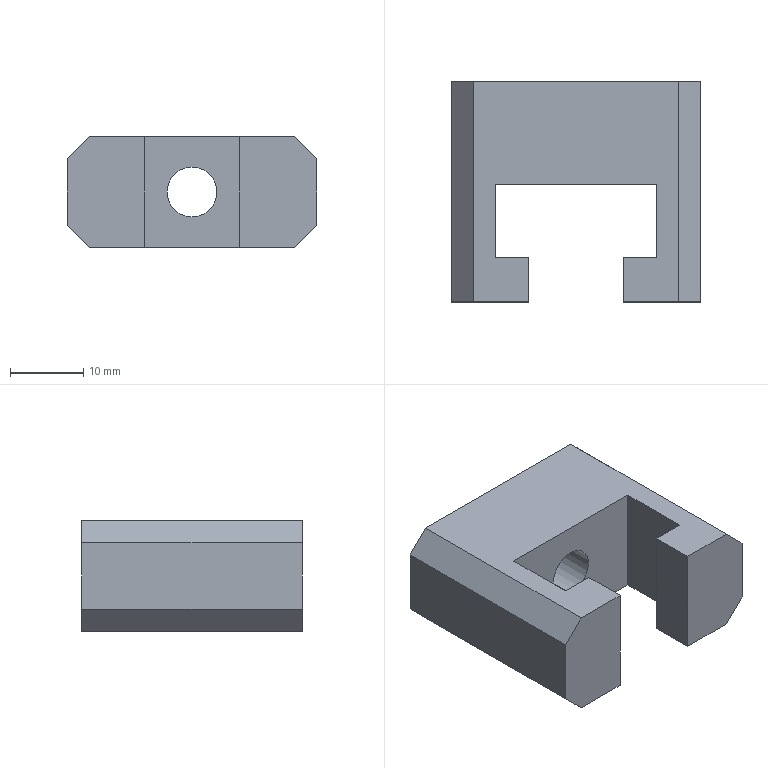Part | STEP file | union 1 | 1 solid | 20 faces | box 34 x 30 x 15 mm | volume 9782 mm3 | plane 18 | cylinder 2 | commonest cylinder face diameters 6.8 x2
STEP:
#1=CARTESIAN_POINT('',(0.,0.,0.));
#2=DIRECTION('',(0.,0.,1.));
#3=DIRECTION('',(1.,0.,0.));
#4=AXIS2_PLACEMENT_3D('',#1,#2,#3);
#5=CARTESIAN_POINT('',(17.,16.,10.9));
#6=VERTEX_POINT('',#5);
#7=CARTESIAN_POINT('',(17.,30.,10.9));
#8=VERTEX_POINT('',#7);
#9=CARTESIAN_POINT('',(17.,30.,10.9));
#10=DIRECTION('',(0.,1.,0.));
#11=VECTOR('',#10,1.);
#12=LINE('',#9,#11);
#13=CARTESIAN_POINT('',(17.,30.,7.5));
#14=DIRECTION('',(0.,1.,0.));
#15=DIRECTION('',(0.,0.,1.));
#16=AXIS2_PLACEMENT_3D('',#13,#14,#15);
#17=CYLINDRICAL_SURFACE('',#16,3.4);
#18=CARTESIAN_POINT('',(6.283,0.));
#19=DIRECTION('',(0.,1.));
#20=VECTOR('',#19,1.);
#21=LINE('',#18,#20);
#22=(GEOMETRIC_REPRESENTATION_CONTEXT(2)PARAMETRIC_REPRESENTATION_CONTEXT()REPRESENTATION_CONTEXT('',''));
#23=DEFINITIONAL_REPRESENTATION('',(#21),#22);
#24=PCURVE('',#17,#23);
#25=CARTESIAN_POINT('',(17.,30.,7.5));
#26=DIRECTION('',(0.,1.,0.));
#27=DIRECTION('',(0.,0.,1.));
#28=AXIS2_PLACEMENT_3D('',#25,#26,#27);
#29=CYLINDRICAL_SURFACE('',#28,3.4);
#30=CARTESIAN_POINT('',(0.,0.));
#31=DIRECTION('',(0.,1.));
#32=VECTOR('',#31,1.);
#33=LINE('',#30,#32);
#34=(GEOMETRIC_REPRESENTATION_CONTEXT(2)PARAMETRIC_REPRESENTATION_CONTEXT()REPRESENTATION_CONTEXT('',''));
#35=DEFINITIONAL_REPRESENTATION('',(#33),#34);
#36=PCURVE('',#29,#35);
#37=SURFACE_CURVE('',#12,(#24,#36),.PCURVE_S1.);
#38=EDGE_CURVE('',#6,#8,#37,.T.);
#39=ORIENTED_EDGE('',*,*,#38,.T.);
#40=CARTESIAN_POINT('',(17.,30.,4.1));
#41=VERTEX_POINT('',#40);
#42=CARTESIAN_POINT('',(17.,30.,7.5));
#43=DIRECTION('',(0.,1.,0.));
#44=DIRECTION('',(0.,0.,1.));
#45=AXIS2_PLACEMENT_3D('',#42,#43,#44);
#46=CIRCLE('',#45,3.4);
#47=CARTESIAN_POINT('',(0.,0.));
#48=DIRECTION('',(1.,0.));
#49=VECTOR('',#48,1.);
#50=LINE('',#47,#49);
#51=(GEOMETRIC_REPRESENTATION_CONTEXT(2)PARAMETRIC_REPRESENTATION_CONTEXT()REPRESENTATION_CONTEXT('',''));
#52=DEFINITIONAL_REPRESENTATION('',(#50),#51);
#53=PCURVE('',#17,#52);
#54=CARTESIAN_POINT('',(0.,30.,15.));
#55=DIRECTION('',(0.,-1.,0.));
#56=DIRECTION('',(1.,0.,0.));
#57=AXIS2_PLACEMENT_3D('',#54,#55,#56);
#58=PLANE('',#57);
#59=CARTESIAN_POINT('',(17.,-4.1));
#60=CARTESIAN_POINT('',(22.889,-4.1));
#61=CARTESIAN_POINT('',(19.944,-9.2));
#62=CARTESIAN_POINT('',(17.,-14.3));
#63=CARTESIAN_POINT('',(14.056,-9.2));
#64=CARTESIAN_POINT('',(11.111,-4.1));
#65=CARTESIAN_POINT('',(17.,-4.1));
#66=(BOUNDED_CURVE()B_SPLINE_CURVE(2,(#59,#60,#61,#62,#63,#64,#65),.UNSPECIFIED.,.T.,.F.)B_SPLINE_CURVE_WITH_KNOTS((1,2,2,2,2,1),(-2.094,0.,2.094,4.189,6.283,8.378),.UNSPECIFIED.)CURVE()GEOMETRIC_REPRESENTATION_ITEM()RATIONAL_B_SPLINE_CURVE((1.,0.5,1.,0.5,1.,0.5,1.))REPRESENTATION_ITEM(''));
#67=(GEOMETRIC_REPRESENTATION_CONTEXT(2)PARAMETRIC_REPRESENTATION_CONTEXT()REPRESENTATION_CONTEXT('',''));
#68=DEFINITIONAL_REPRESENTATION('',(#66),#67);
#69=PCURVE('',#58,#68);
#70=SURFACE_CURVE('',#46,(#53,#69),.PCURVE_S1.);
#71=EDGE_CURVE('',#41,#8,#70,.T.);
#72=ORIENTED_EDGE('',*,*,#71,.F.);
#73=CARTESIAN_POINT('',(17.,16.,4.1));
#74=VERTEX_POINT('',#73);
#75=CARTESIAN_POINT('',(17.,30.,4.1));
#76=DIRECTION('',(0.,1.,0.));
#77=VECTOR('',#76,1.);
#78=LINE('',#75,#77);
#79=CARTESIAN_POINT('',(3.142,0.));
#80=DIRECTION('',(0.,1.));
#81=VECTOR('',#80,1.);
#82=LINE('',#79,#81);
#83=(GEOMETRIC_REPRESENTATION_CONTEXT(2)PARAMETRIC_REPRESENTATION_CONTEXT()REPRESENTATION_CONTEXT('',''));
#84=DEFINITIONAL_REPRESENTATION('',(#82),#83);
#85=PCURVE('',#17,#84);
#86=CARTESIAN_POINT('',(3.142,0.));
#87=DIRECTION('',(0.,1.));
#88=VECTOR('',#87,1.);
#89=LINE('',#86,#88);
#90=(GEOMETRIC_REPRESENTATION_CONTEXT(2)PARAMETRIC_REPRESENTATION_CONTEXT()REPRESENTATION_CONTEXT('',''));
#91=DEFINITIONAL_REPRESENTATION('',(#89),#90);
#92=PCURVE('',#29,#91);
#93=SURFACE_CURVE('',#78,(#85,#92),.PCURVE_S1.);
#94=EDGE_CURVE('',#74,#41,#93,.T.);
#95=ORIENTED_EDGE('',*,*,#94,.F.);
#96=CARTESIAN_POINT('',(17.,16.,7.5));
#97=DIRECTION('',(0.,1.,0.));
#98=DIRECTION('',(-1.,0.,0.));
#99=AXIS2_PLACEMENT_3D('',#96,#97,#98);
#100=CIRCLE('',#99,3.4);
#101=CARTESIAN_POINT('',(-1.571,-14.));
#102=DIRECTION('',(1.,0.));
#103=VECTOR('',#102,1.);
#104=LINE('',#101,#103);
#105=(GEOMETRIC_REPRESENTATION_CONTEXT(2)PARAMETRIC_REPRESENTATION_CONTEXT()REPRESENTATION_CONTEXT('',''));
#106=DEFINITIONAL_REPRESENTATION('',(#104),#105);
#107=PCURVE('',#17,#106);
#108=CARTESIAN_POINT('',(6.,16.,15.));
#109=DIRECTION('',(0.,1.,0.));
#110=DIRECTION('',(-1.,0.,0.));
#111=AXIS2_PLACEMENT_3D('',#108,#109,#110);
#112=PLANE('',#111);
#113=CARTESIAN_POINT('',(-11.,-7.5));
#114=DIRECTION('',(1.,0.));
#115=AXIS2_PLACEMENT_2D('',#113,#114);
#116=CIRCLE('',#115,3.4);
#117=(GEOMETRIC_REPRESENTATION_CONTEXT(2)PARAMETRIC_REPRESENTATION_CONTEXT()REPRESENTATION_CONTEXT('',''));
#118=DEFINITIONAL_REPRESENTATION('',(#116),#117);
#119=PCURVE('',#112,#118);
#120=SURFACE_CURVE('',#100,(#107,#119),.PCURVE_S1.);
#121=EDGE_CURVE('',#74,#6,#120,.T.);
#122=ORIENTED_EDGE('',*,*,#121,.T.);
#123=EDGE_LOOP('',(#39,#72,#95,#122));
#124=FACE_BOUND('',#123,.F.);
#125=ADVANCED_FACE('',(#124),#17,.F.);
#126=CARTESIAN_POINT('',(0.,30.,12.));
#127=VERTEX_POINT('',#126);
#128=CARTESIAN_POINT('',(0.,30.,3.));
#129=VERTEX_POINT('',#128);
#130=CARTESIAN_POINT('',(0.,30.,15.));
#131=DIRECTION('',(0.,0.,-1.));
#132=VECTOR('',#131,1.);
#133=LINE('',#130,#132);
#134=CARTESIAN_POINT('',(0.,0.));
#135=DIRECTION('',(0.,-1.));
#136=VECTOR('',#135,1.);
#137=LINE('',#134,#136);
#138=(GEOMETRIC_REPRESENTATION_CONTEXT(2)PARAMETRIC_REPRESENTATION_CONTEXT()REPRESENTATION_CONTEXT('',''));
#139=DEFINITIONAL_REPRESENTATION('',(#137),#138);
#140=PCURVE('',#58,#139);
#141=CARTESIAN_POINT('',(0.,0.,15.));
#142=DIRECTION('',(1.,0.,0.));
#143=DIRECTION('',(0.,0.,-1.));
#144=AXIS2_PLACEMENT_3D('',#141,#142,#143);
#145=PLANE('',#144);
#146=CARTESIAN_POINT('',(0.,30.));
#147=DIRECTION('',(1.,0.));
#148=VECTOR('',#147,1.);
#149=LINE('',#146,#148);
#150=(GEOMETRIC_REPRESENTATION_CONTEXT(2)PARAMETRIC_REPRESENTATION_CONTEXT()REPRESENTATION_CONTEXT('',''));
#151=DEFINITIONAL_REPRESENTATION('',(#149),#150);
#152=PCURVE('',#145,#151);
#153=SURFACE_CURVE('',#133,(#140,#152),.PCURVE_S1.);
#154=EDGE_CURVE('',#127,#129,#153,.T.);
#155=ORIENTED_EDGE('',*,*,#154,.F.);
#156=CARTESIAN_POINT('',(3.,30.,15.));
#157=VERTEX_POINT('',#156);
#158=CARTESIAN_POINT('',(3.,30.,15.));
#159=DIRECTION('',(0.7071,0.,0.7071));
#160=VECTOR('',#159,1.);
#161=LINE('',#158,#160);
#162=CARTESIAN_POINT('',(3.,0.));
#163=DIRECTION('',(0.7071,0.7071));
#164=VECTOR('',#163,1.);
#165=LINE('',#162,#164);
#166=(GEOMETRIC_REPRESENTATION_CONTEXT(2)PARAMETRIC_REPRESENTATION_CONTEXT()REPRESENTATION_CONTEXT('',''));
#167=DEFINITIONAL_REPRESENTATION('',(#165),#166);
#168=PCURVE('',#58,#167);
#169=CARTESIAN_POINT('',(3.,0.,15.));
#170=DIRECTION('',(0.7071,0.,-0.7071));
#171=DIRECTION('',(-0.7071,0.,-0.7071));
#172=AXIS2_PLACEMENT_3D('',#169,#170,#171);
#173=PLANE('',#172);
#174=CARTESIAN_POINT('',(0.,30.));
#175=DIRECTION('',(-1.,0.));
#176=VECTOR('',#175,1.);
#177=LINE('',#174,#176);
#178=(GEOMETRIC_REPRESENTATION_CONTEXT(2)PARAMETRIC_REPRESENTATION_CONTEXT()REPRESENTATION_CONTEXT('',''));
#179=DEFINITIONAL_REPRESENTATION('',(#177),#178);
#180=PCURVE('',#173,#179);
#181=SURFACE_CURVE('',#161,(#168,#180),.PCURVE_S1.);
#182=EDGE_CURVE('',#127,#157,#181,.T.);
#183=ORIENTED_EDGE('',*,*,#182,.T.);
#184=CARTESIAN_POINT('',(31.,30.,15.));
#185=VERTEX_POINT('',#184);
#186=CARTESIAN_POINT('',(0.,30.,15.));
#187=DIRECTION('',(-1.,0.,0.));
#188=VECTOR('',#187,1.);
#189=LINE('',#186,#188);
#190=CARTESIAN_POINT('',(0.,0.));
#191=DIRECTION('',(-1.,0.));
#192=VECTOR('',#191,1.);
#193=LINE('',#190,#192);
#194=(GEOMETRIC_REPRESENTATION_CONTEXT(2)PARAMETRIC_REPRESENTATION_CONTEXT()REPRESENTATION_CONTEXT('',''));
#195=DEFINITIONAL_REPRESENTATION('',(#193),#194);
#196=PCURVE('',#58,#195);
#197=CARTESIAN_POINT('',(0.,0.,15.));
#198=DIRECTION('',(0.,0.,-1.));
#199=DIRECTION('',(-1.,0.,0.));
#200=AXIS2_PLACEMENT_3D('',#197,#198,#199);
#201=PLANE('',#200);
#202=CARTESIAN_POINT('',(0.,30.));
#203=DIRECTION('',(1.,0.));
#204=VECTOR('',#203,1.);
#205=LINE('',#202,#204);
#206=(GEOMETRIC_REPRESENTATION_CONTEXT(2)PARAMETRIC_REPRESENTATION_CONTEXT()REPRESENTATION_CONTEXT('',''));
#207=DEFINITIONAL_REPRESENTATION('',(#205),#206);
#208=PCURVE('',#201,#207);
#209=SURFACE_CURVE('',#189,(#196,#208),.PCURVE_S1.);
#210=EDGE_CURVE('',#185,#157,#209,.T.);
#211=ORIENTED_EDGE('',*,*,#210,.F.);
#212=CARTESIAN_POINT('',(34.,30.,12.));
#213=VERTEX_POINT('',#212);
#214=CARTESIAN_POINT('',(31.,30.,15.));
#215=DIRECTION('',(0.7071,0.,-0.7071));
#216=VECTOR('',#215,1.);
#217=LINE('',#214,#216);
#218=CARTESIAN_POINT('',(31.,0.));
#219=DIRECTION('',(0.7071,-0.7071));
#220=VECTOR('',#219,1.);
#221=LINE('',#218,#220);
#222=(GEOMETRIC_REPRESENTATION_CONTEXT(2)PARAMETRIC_REPRESENTATION_CONTEXT()REPRESENTATION_CONTEXT('',''));
#223=DEFINITIONAL_REPRESENTATION('',(#221),#222);
#224=PCURVE('',#58,#223);
#225=CARTESIAN_POINT('',(31.,0.,15.));
#226=DIRECTION('',(-0.7071,0.,-0.7071));
#227=DIRECTION('',(-0.7071,0.,0.7071));
#228=AXIS2_PLACEMENT_3D('',#225,#226,#227);
#229=PLANE('',#228);
#230=CARTESIAN_POINT('',(0.,30.));
#231=DIRECTION('',(-1.,0.));
#232=VECTOR('',#231,1.);
#233=LINE('',#230,#232);
#234=(GEOMETRIC_REPRESENTATION_CONTEXT(2)PARAMETRIC_REPRESENTATION_CONTEXT()REPRESENTATION_CONTEXT('',''));
#235=DEFINITIONAL_REPRESENTATION('',(#233),#234);
#236=PCURVE('',#229,#235);
#237=SURFACE_CURVE('',#217,(#224,#236),.PCURVE_S1.);
#238=EDGE_CURVE('',#185,#213,#237,.T.);
#239=ORIENTED_EDGE('',*,*,#238,.T.);
#240=CARTESIAN_POINT('',(34.,30.,3.));
#241=VERTEX_POINT('',#240);
#242=CARTESIAN_POINT('',(34.,30.,15.));
#243=DIRECTION('',(0.,0.,-1.));
#244=VECTOR('',#243,1.);
#245=LINE('',#242,#244);
#246=CARTESIAN_POINT('',(34.,0.));
#247=DIRECTION('',(0.,-1.));
#248=VECTOR('',#247,1.);
#249=LINE('',#246,#248);
#250=(GEOMETRIC_REPRESENTATION_CONTEXT(2)PARAMETRIC_REPRESENTATION_CONTEXT()REPRESENTATION_CONTEXT('',''));
#251=DEFINITIONAL_REPRESENTATION('',(#249),#250);
#252=PCURVE('',#58,#251);
#253=CARTESIAN_POINT('',(34.,0.,15.));
#254=DIRECTION('',(-1.,0.,0.));
#255=DIRECTION('',(0.,-1.,0.));
#256=AXIS2_PLACEMENT_3D('',#253,#254,#255);
#257=PLANE('',#256);
#258=CARTESIAN_POINT('',(-30.,0.));
#259=DIRECTION('',(0.,-1.));
#260=VECTOR('',#259,1.);
#261=LINE('',#258,#260);
#262=(GEOMETRIC_REPRESENTATION_CONTEXT(2)PARAMETRIC_REPRESENTATION_CONTEXT()REPRESENTATION_CONTEXT('',''));
#263=DEFINITIONAL_REPRESENTATION('',(#261),#262);
#264=PCURVE('',#257,#263);
#265=SURFACE_CURVE('',#245,(#252,#264),.PCURVE_S1.);
#266=EDGE_CURVE('',#213,#241,#265,.T.);
#267=ORIENTED_EDGE('',*,*,#266,.T.);
#268=CARTESIAN_POINT('',(31.,30.,0.));
#269=VERTEX_POINT('',#268);
#270=CARTESIAN_POINT('',(34.,30.,3.));
#271=DIRECTION('',(-0.7071,0.,-0.7071));
#272=VECTOR('',#271,1.);
#273=LINE('',#270,#272);
#274=CARTESIAN_POINT('',(34.,-12.));
#275=DIRECTION('',(-0.7071,-0.7071));
#276=VECTOR('',#275,1.);
#277=LINE('',#274,#276);
#278=(GEOMETRIC_REPRESENTATION_CONTEXT(2)PARAMETRIC_REPRESENTATION_CONTEXT()REPRESENTATION_CONTEXT('',''));
#279=DEFINITIONAL_REPRESENTATION('',(#277),#278);
#280=PCURVE('',#58,#279);
#281=CARTESIAN_POINT('',(34.,0.,3.));
#282=DIRECTION('',(0.7071,0.,-0.7071));
#283=DIRECTION('',(-0.7071,0.,-0.7071));
#284=AXIS2_PLACEMENT_3D('',#281,#282,#283);
#285=PLANE('',#284);
#286=CARTESIAN_POINT('',(0.,30.));
#287=DIRECTION('',(1.,0.));
#288=VECTOR('',#287,1.);
#289=LINE('',#286,#288);
#290=(GEOMETRIC_REPRESENTATION_CONTEXT(2)PARAMETRIC_REPRESENTATION_CONTEXT()REPRESENTATION_CONTEXT('',''));
#291=DEFINITIONAL_REPRESENTATION('',(#289),#290);
#292=PCURVE('',#285,#291);
#293=SURFACE_CURVE('',#273,(#280,#292),.PCURVE_S1.);
#294=EDGE_CURVE('',#241,#269,#293,.T.);
#295=ORIENTED_EDGE('',*,*,#294,.T.);
#296=CARTESIAN_POINT('',(3.,30.,0.));
#297=VERTEX_POINT('',#296);
#298=CARTESIAN_POINT('',(0.,30.,0.));
#299=DIRECTION('',(-1.,0.,0.));
#300=VECTOR('',#299,1.);
#301=LINE('',#298,#300);
#302=CARTESIAN_POINT('',(0.,-15.));
#303=DIRECTION('',(-1.,0.));
#304=VECTOR('',#303,1.);
#305=LINE('',#302,#304);
#306=(GEOMETRIC_REPRESENTATION_CONTEXT(2)PARAMETRIC_REPRESENTATION_CONTEXT()REPRESENTATION_CONTEXT('',''));
#307=DEFINITIONAL_REPRESENTATION('',(#305),#306);
#308=PCURVE('',#58,#307);
#309=CARTESIAN_POINT('',(0.,0.,0.));
#310=DIRECTION('',(0.,0.,-1.));
#311=DIRECTION('',(-1.,0.,0.));
#312=AXIS2_PLACEMENT_3D('',#309,#310,#311);
#313=PLANE('',#312);
#314=CARTESIAN_POINT('',(0.,30.));
#315=DIRECTION('',(1.,0.));
#316=VECTOR('',#315,1.);
#317=LINE('',#314,#316);
#318=(GEOMETRIC_REPRESENTATION_CONTEXT(2)PARAMETRIC_REPRESENTATION_CONTEXT()REPRESENTATION_CONTEXT('',''));
#319=DEFINITIONAL_REPRESENTATION('',(#317),#318);
#320=PCURVE('',#313,#319);
#321=SURFACE_CURVE('',#301,(#308,#320),.PCURVE_S1.);
#322=EDGE_CURVE('',#269,#297,#321,.T.);
#323=ORIENTED_EDGE('',*,*,#322,.T.);
#324=CARTESIAN_POINT('',(0.,30.,3.));
#325=DIRECTION('',(-0.7071,0.,0.7071));
#326=VECTOR('',#325,1.);
#327=LINE('',#324,#326);
#328=CARTESIAN_POINT('',(0.,-12.));
#329=DIRECTION('',(-0.7071,0.7071));
#330=VECTOR('',#329,1.);
#331=LINE('',#328,#330);
#332=(GEOMETRIC_REPRESENTATION_CONTEXT(2)PARAMETRIC_REPRESENTATION_CONTEXT()REPRESENTATION_CONTEXT('',''));
#333=DEFINITIONAL_REPRESENTATION('',(#331),#332);
#334=PCURVE('',#58,#333);
#335=CARTESIAN_POINT('',(0.,0.,3.));
#336=DIRECTION('',(-0.7071,0.,-0.7071));
#337=DIRECTION('',(-0.7071,0.,0.7071));
#338=AXIS2_PLACEMENT_3D('',#335,#336,#337);
#339=PLANE('',#338);
#340=CARTESIAN_POINT('',(0.,30.));
#341=DIRECTION('',(1.,0.));
#342=VECTOR('',#341,1.);
#343=LINE('',#340,#342);
#344=(GEOMETRIC_REPRESENTATION_CONTEXT(2)PARAMETRIC_REPRESENTATION_CONTEXT()REPRESENTATION_CONTEXT('',''));
#345=DEFINITIONAL_REPRESENTATION('',(#343),#344);
#346=PCURVE('',#339,#345);
#347=SURFACE_CURVE('',#327,(#334,#346),.PCURVE_S1.);
#348=EDGE_CURVE('',#297,#129,#347,.T.);
#349=ORIENTED_EDGE('',*,*,#348,.T.);
#350=EDGE_LOOP('',(#155,#183,#211,#239,#267,#295,#323,#349));
#351=FACE_BOUND('',#350,.T.);
#352=CARTESIAN_POINT('',(17.,30.,7.5));
#353=DIRECTION('',(0.,1.,0.));
#354=DIRECTION('',(0.,0.,1.));
#355=AXIS2_PLACEMENT_3D('',#352,#353,#354);
#356=CIRCLE('',#355,3.4);
#357=CARTESIAN_POINT('',(17.,-4.1));
#358=CARTESIAN_POINT('',(22.889,-4.1));
#359=CARTESIAN_POINT('',(19.944,-9.2));
#360=CARTESIAN_POINT('',(17.,-14.3));
#361=CARTESIAN_POINT('',(14.056,-9.2));
#362=CARTESIAN_POINT('',(11.111,-4.1));
#363=CARTESIAN_POINT('',(17.,-4.1));
#364=(BOUNDED_CURVE()B_SPLINE_CURVE(2,(#357,#358,#359,#360,#361,#362,#363),.UNSPECIFIED.,.T.,.F.)B_SPLINE_CURVE_WITH_KNOTS((1,2,2,2,2,1),(-2.094,0.,2.094,4.189,6.283,8.378),.UNSPECIFIED.)CURVE()GEOMETRIC_REPRESENTATION_ITEM()RATIONAL_B_SPLINE_CURVE((1.,0.5,1.,0.5,1.,0.5,1.))REPRESENTATION_ITEM(''));
#365=(GEOMETRIC_REPRESENTATION_CONTEXT(2)PARAMETRIC_REPRESENTATION_CONTEXT()REPRESENTATION_CONTEXT('',''));
#366=DEFINITIONAL_REPRESENTATION('',(#364),#365);
#367=PCURVE('',#58,#366);
#368=CARTESIAN_POINT('',(0.,0.));
#369=DIRECTION('',(1.,0.));
#370=VECTOR('',#369,1.);
#371=LINE('',#368,#370);
#372=(GEOMETRIC_REPRESENTATION_CONTEXT(2)PARAMETRIC_REPRESENTATION_CONTEXT()REPRESENTATION_CONTEXT('',''));
#373=DEFINITIONAL_REPRESENTATION('',(#371),#372);
#374=PCURVE('',#29,#373);
#375=SURFACE_CURVE('',#356,(#367,#374),.PCURVE_S1.);
#376=EDGE_CURVE('',#8,#41,#375,.T.);
#377=ORIENTED_EDGE('',*,*,#376,.F.);
#378=ORIENTED_EDGE('',*,*,#71,.F.);
#379=EDGE_LOOP('',(#377,#378));
#380=FACE_BOUND('',#379,.T.);
#381=ADVANCED_FACE('',(#351,#380),#58,.F.);
#382=CARTESIAN_POINT('',(0.,0.,12.));
#383=VERTEX_POINT('',#382);
#384=CARTESIAN_POINT('',(0.,0.,3.));
#385=VERTEX_POINT('',#384);
#386=CARTESIAN_POINT('',(0.,0.,15.));
#387=DIRECTION('',(0.,0.,-1.));
#388=VECTOR('',#387,1.);
#389=LINE('',#386,#388);
#390=CARTESIAN_POINT('',(0.,0.));
#391=DIRECTION('',(1.,0.));
#392=VECTOR('',#391,1.);
#393=LINE('',#390,#392);
#394=(GEOMETRIC_REPRESENTATION_CONTEXT(2)PARAMETRIC_REPRESENTATION_CONTEXT()REPRESENTATION_CONTEXT('',''));
#395=DEFINITIONAL_REPRESENTATION('',(#393),#394);
#396=PCURVE('',#145,#395);
#397=CARTESIAN_POINT('',(0.,0.,15.));
#398=DIRECTION('',(0.,1.,0.));
#399=DIRECTION('',(0.,0.,1.));
#400=AXIS2_PLACEMENT_3D('',#397,#398,#399);
#401=PLANE('',#400);
#402=CARTESIAN_POINT('',(0.,0.));
#403=DIRECTION('',(-1.,0.));
#404=VECTOR('',#403,1.);
#405=LINE('',#402,#404);
#406=(GEOMETRIC_REPRESENTATION_CONTEXT(2)PARAMETRIC_REPRESENTATION_CONTEXT()REPRESENTATION_CONTEXT('',''));
#407=DEFINITIONAL_REPRESENTATION('',(#405),#406);
#408=PCURVE('',#401,#407);
#409=SURFACE_CURVE('',#389,(#396,#408),.PCURVE_S1.);
#410=EDGE_CURVE('',#383,#385,#409,.T.);
#411=ORIENTED_EDGE('',*,*,#410,.F.);
#412=CARTESIAN_POINT('',(0.,0.,12.));
#413=DIRECTION('',(0.,1.,0.));
#414=VECTOR('',#413,1.);
#415=LINE('',#412,#414);
#416=CARTESIAN_POINT('',(3.,0.));
#417=DIRECTION('',(0.,1.));
#418=VECTOR('',#417,1.);
#419=LINE('',#416,#418);
#420=(GEOMETRIC_REPRESENTATION_CONTEXT(2)PARAMETRIC_REPRESENTATION_CONTEXT()REPRESENTATION_CONTEXT('',''));
#421=DEFINITIONAL_REPRESENTATION('',(#419),#420);
#422=PCURVE('',#145,#421);
#423=CARTESIAN_POINT('',(4.243,0.));
#424=DIRECTION('',(0.,1.));
#425=VECTOR('',#424,1.);
#426=LINE('',#423,#425);
#427=(GEOMETRIC_REPRESENTATION_CONTEXT(2)PARAMETRIC_REPRESENTATION_CONTEXT()REPRESENTATION_CONTEXT('',''));
#428=DEFINITIONAL_REPRESENTATION('',(#426),#427);
#429=PCURVE('',#173,#428);
#430=SURFACE_CURVE('',#415,(#422,#429),.PCURVE_S1.);
#431=EDGE_CURVE('',#383,#127,#430,.T.);
#432=ORIENTED_EDGE('',*,*,#431,.T.);
#433=ORIENTED_EDGE('',*,*,#154,.T.);
#434=CARTESIAN_POINT('',(0.,0.,3.));
#435=DIRECTION('',(0.,-1.,0.));
#436=VECTOR('',#435,1.);
#437=LINE('',#434,#436);
#438=CARTESIAN_POINT('',(12.,0.));
#439=DIRECTION('',(0.,-1.));
#440=VECTOR('',#439,1.);
#441=LINE('',#438,#440);
#442=(GEOMETRIC_REPRESENTATION_CONTEXT(2)PARAMETRIC_REPRESENTATION_CONTEXT()REPRESENTATION_CONTEXT('',''));
#443=DEFINITIONAL_REPRESENTATION('',(#441),#442);
#444=PCURVE('',#145,#443);
#445=CARTESIAN_POINT('',(0.,0.));
#446=DIRECTION('',(0.,-1.));
#447=VECTOR('',#446,1.);
#448=LINE('',#445,#447);
#449=(GEOMETRIC_REPRESENTATION_CONTEXT(2)PARAMETRIC_REPRESENTATION_CONTEXT()REPRESENTATION_CONTEXT('',''));
#450=DEFINITIONAL_REPRESENTATION('',(#448),#449);
#451=PCURVE('',#339,#450);
#452=SURFACE_CURVE('',#437,(#444,#451),.PCURVE_S1.);
#453=EDGE_CURVE('',#129,#385,#452,.T.);
#454=ORIENTED_EDGE('',*,*,#453,.T.);
#455=EDGE_LOOP('',(#411,#432,#433,#454));
#456=FACE_BOUND('',#455,.T.);
#457=ADVANCED_FACE('',(#456),#145,.F.);
#458=CARTESIAN_POINT('',(3.,0.,15.));
#459=VERTEX_POINT('',#458);
#460=CARTESIAN_POINT('',(10.5,0.,15.));
#461=VERTEX_POINT('',#460);
#462=CARTESIAN_POINT('',(0.,0.,15.));
#463=DIRECTION('',(1.,0.,0.));
#464=VECTOR('',#463,1.);
#465=LINE('',#462,#464);
#466=CARTESIAN_POINT('',(0.,0.));
#467=DIRECTION('',(0.,1.));
#468=VECTOR('',#467,1.);
#469=LINE('',#466,#468);
#470=(GEOMETRIC_REPRESENTATION_CONTEXT(2)PARAMETRIC_REPRESENTATION_CONTEXT()REPRESENTATION_CONTEXT('',''));
#471=DEFINITIONAL_REPRESENTATION('',(#469),#470);
#472=PCURVE('',#401,#471);
#473=CARTESIAN_POINT('',(0.,0.));
#474=DIRECTION('',(-1.,0.));
#475=VECTOR('',#474,1.);
#476=LINE('',#473,#475);
#477=(GEOMETRIC_REPRESENTATION_CONTEXT(2)PARAMETRIC_REPRESENTATION_CONTEXT()REPRESENTATION_CONTEXT('',''));
#478=DEFINITIONAL_REPRESENTATION('',(#476),#477);
#479=PCURVE('',#201,#478);
#480=SURFACE_CURVE('',#465,(#472,#479),.PCURVE_S1.);
#481=EDGE_CURVE('',#459,#461,#480,.T.);
#482=ORIENTED_EDGE('',*,*,#481,.F.);
#483=CARTESIAN_POINT('',(3.,0.,15.));
#484=DIRECTION('',(-0.7071,0.,-0.7071));
#485=VECTOR('',#484,1.);
#486=LINE('',#483,#485);
#487=CARTESIAN_POINT('',(0.,3.));
#488=DIRECTION('',(-0.7071,-0.7071));
#489=VECTOR('',#488,1.);
#490=LINE('',#487,#489);
#491=(GEOMETRIC_REPRESENTATION_CONTEXT(2)PARAMETRIC_REPRESENTATION_CONTEXT()REPRESENTATION_CONTEXT('',''));
#492=DEFINITIONAL_REPRESENTATION('',(#490),#491);
#493=PCURVE('',#401,#492);
#494=CARTESIAN_POINT('',(0.,0.));
#495=DIRECTION('',(1.,0.));
#496=VECTOR('',#495,1.);
#497=LINE('',#494,#496);
#498=(GEOMETRIC_REPRESENTATION_CONTEXT(2)PARAMETRIC_REPRESENTATION_CONTEXT()REPRESENTATION_CONTEXT('',''));
#499=DEFINITIONAL_REPRESENTATION('',(#497),#498);
#500=PCURVE('',#173,#499);
#501=SURFACE_CURVE('',#486,(#493,#500),.PCURVE_S1.);
#502=EDGE_CURVE('',#459,#383,#501,.T.);
#503=ORIENTED_EDGE('',*,*,#502,.T.);
#504=ORIENTED_EDGE('',*,*,#410,.T.);
#505=CARTESIAN_POINT('',(3.,0.,0.));
#506=VERTEX_POINT('',#505);
#507=CARTESIAN_POINT('',(0.,0.,3.));
#508=DIRECTION('',(0.7071,0.,-0.7071));
#509=VECTOR('',#508,1.);
#510=LINE('',#507,#509);
#511=CARTESIAN_POINT('',(-12.,0.));
#512=DIRECTION('',(-0.7071,0.7071));
#513=VECTOR('',#512,1.);
#514=LINE('',#511,#513);
#515=(GEOMETRIC_REPRESENTATION_CONTEXT(2)PARAMETRIC_REPRESENTATION_CONTEXT()REPRESENTATION_CONTEXT('',''));
#516=DEFINITIONAL_REPRESENTATION('',(#514),#515);
#517=PCURVE('',#401,#516);
#518=CARTESIAN_POINT('',(0.,0.));
#519=DIRECTION('',(-1.,0.));
#520=VECTOR('',#519,1.);
#521=LINE('',#518,#520);
#522=(GEOMETRIC_REPRESENTATION_CONTEXT(2)PARAMETRIC_REPRESENTATION_CONTEXT()REPRESENTATION_CONTEXT('',''));
#523=DEFINITIONAL_REPRESENTATION('',(#521),#522);
#524=PCURVE('',#339,#523);
#525=SURFACE_CURVE('',#510,(#517,#524),.PCURVE_S1.);
#526=EDGE_CURVE('',#385,#506,#525,.T.);
#527=ORIENTED_EDGE('',*,*,#526,.T.);
#528=CARTESIAN_POINT('',(10.5,0.,0.));
#529=VERTEX_POINT('',#528);
#530=CARTESIAN_POINT('',(0.,0.,0.));
#531=DIRECTION('',(1.,0.,0.));
#532=VECTOR('',#531,1.);
#533=LINE('',#530,#532);
#534=CARTESIAN_POINT('',(-15.,0.));
#535=DIRECTION('',(0.,1.));
#536=VECTOR('',#535,1.);
#537=LINE('',#534,#536);
#538=(GEOMETRIC_REPRESENTATION_CONTEXT(2)PARAMETRIC_REPRESENTATION_CONTEXT()REPRESENTATION_CONTEXT('',''));
#539=DEFINITIONAL_REPRESENTATION('',(#537),#538);
#540=PCURVE('',#401,#539);
#541=CARTESIAN_POINT('',(0.,0.));
#542=DIRECTION('',(-1.,0.));
#543=VECTOR('',#542,1.);
#544=LINE('',#541,#543);
#545=(GEOMETRIC_REPRESENTATION_CONTEXT(2)PARAMETRIC_REPRESENTATION_CONTEXT()REPRESENTATION_CONTEXT('',''));
#546=DEFINITIONAL_REPRESENTATION('',(#544),#545);
#547=PCURVE('',#313,#546);
#548=SURFACE_CURVE('',#533,(#540,#547),.PCURVE_S1.);
#549=EDGE_CURVE('',#506,#529,#548,.T.);
#550=ORIENTED_EDGE('',*,*,#549,.T.);
#551=CARTESIAN_POINT('',(10.5,0.,15.));
#552=DIRECTION('',(0.,0.,-1.));
#553=VECTOR('',#552,1.);
#554=LINE('',#551,#553);
#555=CARTESIAN_POINT('',(0.,10.5));
#556=DIRECTION('',(-1.,0.));
#557=VECTOR('',#556,1.);
#558=LINE('',#555,#557);
#559=(GEOMETRIC_REPRESENTATION_CONTEXT(2)PARAMETRIC_REPRESENTATION_CONTEXT()REPRESENTATION_CONTEXT('',''));
#560=DEFINITIONAL_REPRESENTATION('',(#558),#559);
#561=PCURVE('',#401,#560);
#562=CARTESIAN_POINT('',(10.5,0.,15.));
#563=DIRECTION('',(-1.,0.,0.));
#564=DIRECTION('',(0.,-1.,0.));
#565=AXIS2_PLACEMENT_3D('',#562,#563,#564);
#566=PLANE('',#565);
#567=CARTESIAN_POINT('',(0.,0.));
#568=DIRECTION('',(0.,-1.));
#569=VECTOR('',#568,1.);
#570=LINE('',#567,#569);
#571=(GEOMETRIC_REPRESENTATION_CONTEXT(2)PARAMETRIC_REPRESENTATION_CONTEXT()REPRESENTATION_CONTEXT('',''));
#572=DEFINITIONAL_REPRESENTATION('',(#570),#571);
#573=PCURVE('',#566,#572);
#574=SURFACE_CURVE('',#554,(#561,#573),.PCURVE_S1.);
#575=EDGE_CURVE('',#461,#529,#574,.T.);
#576=ORIENTED_EDGE('',*,*,#575,.F.);
#577=EDGE_LOOP('',(#482,#503,#504,#527,#550,#576));
#578=FACE_BOUND('',#577,.T.);
#579=ADVANCED_FACE('',(#578),#401,.F.);
#580=CARTESIAN_POINT('',(10.5,6.,0.));
#581=VERTEX_POINT('',#580);
#582=CARTESIAN_POINT('',(10.5,0.,0.));
#583=DIRECTION('',(0.,1.,0.));
#584=VECTOR('',#583,1.);
#585=LINE('',#582,#584);
#586=CARTESIAN_POINT('',(0.,-15.));
#587=DIRECTION('',(-1.,0.));
#588=VECTOR('',#587,1.);
#589=LINE('',#586,#588);
#590=(GEOMETRIC_REPRESENTATION_CONTEXT(2)PARAMETRIC_REPRESENTATION_CONTEXT()REPRESENTATION_CONTEXT('',''));
#591=DEFINITIONAL_REPRESENTATION('',(#589),#590);
#592=PCURVE('',#566,#591);
#593=CARTESIAN_POINT('',(-10.5,0.));
#594=DIRECTION('',(0.,1.));
#595=VECTOR('',#594,1.);
#596=LINE('',#593,#595);
#597=(GEOMETRIC_REPRESENTATION_CONTEXT(2)PARAMETRIC_REPRESENTATION_CONTEXT()REPRESENTATION_CONTEXT('',''));
#598=DEFINITIONAL_REPRESENTATION('',(#596),#597);
#599=PCURVE('',#313,#598);
#600=SURFACE_CURVE('',#585,(#592,#599),.PCURVE_S1.);
#601=EDGE_CURVE('',#529,#581,#600,.T.);
#602=ORIENTED_EDGE('',*,*,#601,.T.);
#603=CARTESIAN_POINT('',(10.5,6.,15.));
#604=VERTEX_POINT('',#603);
#605=CARTESIAN_POINT('',(10.5,6.,15.));
#606=DIRECTION('',(0.,0.,-1.));
#607=VECTOR('',#606,1.);
#608=LINE('',#605,#607);
#609=CARTESIAN_POINT('',(-6.,0.));
#610=DIRECTION('',(0.,-1.));
#611=VECTOR('',#610,1.);
#612=LINE('',#609,#611);
#613=(GEOMETRIC_REPRESENTATION_CONTEXT(2)PARAMETRIC_REPRESENTATION_CONTEXT()REPRESENTATION_CONTEXT('',''));
#614=DEFINITIONAL_REPRESENTATION('',(#612),#613);
#615=PCURVE('',#566,#614);
#616=CARTESIAN_POINT('',(6.,6.,15.));
#617=DIRECTION('',(0.,-1.,0.));
#618=DIRECTION('',(0.,0.,-1.));
#619=AXIS2_PLACEMENT_3D('',#616,#617,#618);
#620=PLANE('',#619);
#621=CARTESIAN_POINT('',(0.,4.5));
#622=DIRECTION('',(1.,0.));
#623=VECTOR('',#622,1.);
#624=LINE('',#621,#623);
#625=(GEOMETRIC_REPRESENTATION_CONTEXT(2)PARAMETRIC_REPRESENTATION_CONTEXT()REPRESENTATION_CONTEXT('',''));
#626=DEFINITIONAL_REPRESENTATION('',(#624),#625);
#627=PCURVE('',#620,#626);
#628=SURFACE_CURVE('',#608,(#615,#627),.PCURVE_S1.);
#629=EDGE_CURVE('',#604,#581,#628,.T.);
#630=ORIENTED_EDGE('',*,*,#629,.F.);
#631=CARTESIAN_POINT('',(10.5,0.,15.));
#632=DIRECTION('',(0.,1.,0.));
#633=VECTOR('',#632,1.);
#634=LINE('',#631,#633);
#635=CARTESIAN_POINT('',(0.,0.));
#636=DIRECTION('',(-1.,0.));
#637=VECTOR('',#636,1.);
#638=LINE('',#635,#637);
#639=(GEOMETRIC_REPRESENTATION_CONTEXT(2)PARAMETRIC_REPRESENTATION_CONTEXT()REPRESENTATION_CONTEXT('',''));
#640=DEFINITIONAL_REPRESENTATION('',(#638),#639);
#641=PCURVE('',#566,#640);
#642=CARTESIAN_POINT('',(-10.5,0.));
#643=DIRECTION('',(0.,1.));
#644=VECTOR('',#643,1.);
#645=LINE('',#642,#644);
#646=(GEOMETRIC_REPRESENTATION_CONTEXT(2)PARAMETRIC_REPRESENTATION_CONTEXT()REPRESENTATION_CONTEXT('',''));
#647=DEFINITIONAL_REPRESENTATION('',(#645),#646);
#648=PCURVE('',#201,#647);
#649=SURFACE_CURVE('',#634,(#641,#648),.PCURVE_S1.);
#650=EDGE_CURVE('',#461,#604,#649,.T.);
#651=ORIENTED_EDGE('',*,*,#650,.F.);
#652=ORIENTED_EDGE('',*,*,#575,.T.);
#653=EDGE_LOOP('',(#602,#630,#651,#652));
#654=FACE_BOUND('',#653,.T.);
#655=ADVANCED_FACE('',(#654),#566,.F.);
#656=CARTESIAN_POINT('',(6.,6.,0.));
#657=VERTEX_POINT('',#656);
#658=CARTESIAN_POINT('',(6.,6.,0.));
#659=DIRECTION('',(-1.,0.,0.));
#660=VECTOR('',#659,1.);
#661=LINE('',#658,#660);
#662=CARTESIAN_POINT('',(15.,0.));
#663=DIRECTION('',(0.,-1.));
#664=VECTOR('',#663,1.);
#665=LINE('',#662,#664);
#666=(GEOMETRIC_REPRESENTATION_CONTEXT(2)PARAMETRIC_REPRESENTATION_CONTEXT()REPRESENTATION_CONTEXT('',''));
#667=DEFINITIONAL_REPRESENTATION('',(#665),#666);
#668=PCURVE('',#620,#667);
#669=CARTESIAN_POINT('',(-6.,6.));
#670=DIRECTION('',(1.,0.));
#671=VECTOR('',#670,1.);
#672=LINE('',#669,#671);
#673=(GEOMETRIC_REPRESENTATION_CONTEXT(2)PARAMETRIC_REPRESENTATION_CONTEXT()REPRESENTATION_CONTEXT('',''));
#674=DEFINITIONAL_REPRESENTATION('',(#672),#673);
#675=PCURVE('',#313,#674);
#676=SURFACE_CURVE('',#661,(#668,#675),.PCURVE_S1.);
#677=EDGE_CURVE('',#581,#657,#676,.T.);
#678=ORIENTED_EDGE('',*,*,#677,.T.);
#679=CARTESIAN_POINT('',(6.,6.,15.));
#680=VERTEX_POINT('',#679);
#681=CARTESIAN_POINT('',(6.,6.,15.));
#682=DIRECTION('',(0.,0.,-1.));
#683=VECTOR('',#682,1.);
#684=LINE('',#681,#683);
#685=CARTESIAN_POINT('',(0.,0.));
#686=DIRECTION('',(1.,0.));
#687=VECTOR('',#686,1.);
#688=LINE('',#685,#687);
#689=(GEOMETRIC_REPRESENTATION_CONTEXT(2)PARAMETRIC_REPRESENTATION_CONTEXT()REPRESENTATION_CONTEXT('',''));
#690=DEFINITIONAL_REPRESENTATION('',(#688),#689);
#691=PCURVE('',#620,#690);
#692=CARTESIAN_POINT('',(6.,6.,15.));
#693=DIRECTION('',(-1.,0.,0.));
#694=DIRECTION('',(0.,-1.,0.));
#695=AXIS2_PLACEMENT_3D('',#692,#693,#694);
#696=PLANE('',#695);
#697=CARTESIAN_POINT('',(0.,0.));
#698=DIRECTION('',(0.,-1.));
#699=VECTOR('',#698,1.);
#700=LINE('',#697,#699);
#701=(GEOMETRIC_REPRESENTATION_CONTEXT(2)PARAMETRIC_REPRESENTATION_CONTEXT()REPRESENTATION_CONTEXT('',''));
#702=DEFINITIONAL_REPRESENTATION('',(#700),#701);
#703=PCURVE('',#696,#702);
#704=SURFACE_CURVE('',#684,(#691,#703),.PCURVE_S1.);
#705=EDGE_CURVE('',#680,#657,#704,.T.);
#706=ORIENTED_EDGE('',*,*,#705,.F.);
#707=CARTESIAN_POINT('',(6.,6.,15.));
#708=DIRECTION('',(-1.,0.,0.));
#709=VECTOR('',#708,1.);
#710=LINE('',#707,#709);
#711=CARTESIAN_POINT('',(0.,0.));
#712=DIRECTION('',(0.,-1.));
#713=VECTOR('',#712,1.);
#714=LINE('',#711,#713);
#715=(GEOMETRIC_REPRESENTATION_CONTEXT(2)PARAMETRIC_REPRESENTATION_CONTEXT()REPRESENTATION_CONTEXT('',''));
#716=DEFINITIONAL_REPRESENTATION('',(#714),#715);
#717=PCURVE('',#620,#716);
#718=CARTESIAN_POINT('',(-6.,6.));
#719=DIRECTION('',(1.,0.));
#720=VECTOR('',#719,1.);
#721=LINE('',#718,#720);
#722=(GEOMETRIC_REPRESENTATION_CONTEXT(2)PARAMETRIC_REPRESENTATION_CONTEXT()REPRESENTATION_CONTEXT('',''));
#723=DEFINITIONAL_REPRESENTATION('',(#721),#722);
#724=PCURVE('',#201,#723);
#725=SURFACE_CURVE('',#710,(#717,#724),.PCURVE_S1.);
#726=EDGE_CURVE('',#604,#680,#725,.T.);
#727=ORIENTED_EDGE('',*,*,#726,.F.);
#728=ORIENTED_EDGE('',*,*,#629,.T.);
#729=EDGE_LOOP('',(#678,#706,#727,#728));
#730=FACE_BOUND('',#729,.T.);
#731=ADVANCED_FACE('',(#730),#620,.F.);
#732=CARTESIAN_POINT('',(6.,16.,0.));
#733=VERTEX_POINT('',#732);
#734=CARTESIAN_POINT('',(6.,6.,0.));
#735=DIRECTION('',(0.,1.,0.));
#736=VECTOR('',#735,1.);
#737=LINE('',#734,#736);
#738=CARTESIAN_POINT('',(0.,-15.));
#739=DIRECTION('',(-1.,0.));
#740=VECTOR('',#739,1.);
#741=LINE('',#738,#740);
#742=(GEOMETRIC_REPRESENTATION_CONTEXT(2)PARAMETRIC_REPRESENTATION_CONTEXT()REPRESENTATION_CONTEXT('',''));
#743=DEFINITIONAL_REPRESENTATION('',(#741),#742);
#744=PCURVE('',#696,#743);
#745=CARTESIAN_POINT('',(-6.,6.));
#746=DIRECTION('',(0.,1.));
#747=VECTOR('',#746,1.);
#748=LINE('',#745,#747);
#749=(GEOMETRIC_REPRESENTATION_CONTEXT(2)PARAMETRIC_REPRESENTATION_CONTEXT()REPRESENTATION_CONTEXT('',''));
#750=DEFINITIONAL_REPRESENTATION('',(#748),#749);
#751=PCURVE('',#313,#750);
#752=SURFACE_CURVE('',#737,(#744,#751),.PCURVE_S1.);
#753=EDGE_CURVE('',#657,#733,#752,.T.);
#754=ORIENTED_EDGE('',*,*,#753,.T.);
#755=CARTESIAN_POINT('',(6.,16.,15.));
#756=VERTEX_POINT('',#755);
#757=CARTESIAN_POINT('',(6.,16.,15.));
#758=DIRECTION('',(0.,0.,-1.));
#759=VECTOR('',#758,1.);
#760=LINE('',#757,#759);
#761=CARTESIAN_POINT('',(-10.,0.));
#762=DIRECTION('',(0.,-1.));
#763=VECTOR('',#762,1.);
#764=LINE('',#761,#763);
#765=(GEOMETRIC_REPRESENTATION_CONTEXT(2)PARAMETRIC_REPRESENTATION_CONTEXT()REPRESENTATION_CONTEXT('',''));
#766=DEFINITIONAL_REPRESENTATION('',(#764),#765);
#767=PCURVE('',#696,#766);
#768=CARTESIAN_POINT('',(0.,0.));
#769=DIRECTION('',(0.,-1.));
#770=VECTOR('',#769,1.);
#771=LINE('',#768,#770);
#772=(GEOMETRIC_REPRESENTATION_CONTEXT(2)PARAMETRIC_REPRESENTATION_CONTEXT()REPRESENTATION_CONTEXT('',''));
#773=DEFINITIONAL_REPRESENTATION('',(#771),#772);
#774=PCURVE('',#112,#773);
#775=SURFACE_CURVE('',#760,(#767,#774),.PCURVE_S1.);
#776=EDGE_CURVE('',#756,#733,#775,.T.);
#777=ORIENTED_EDGE('',*,*,#776,.F.);
#778=CARTESIAN_POINT('',(6.,6.,15.));
#779=DIRECTION('',(0.,1.,0.));
#780=VECTOR('',#779,1.);
#781=LINE('',#778,#780);
#782=CARTESIAN_POINT('',(0.,0.));
#783=DIRECTION('',(-1.,0.));
#784=VECTOR('',#783,1.);
#785=LINE('',#782,#784);
#786=(GEOMETRIC_REPRESENTATION_CONTEXT(2)PARAMETRIC_REPRESENTATION_CONTEXT()REPRESENTATION_CONTEXT('',''));
#787=DEFINITIONAL_REPRESENTATION('',(#785),#786);
#788=PCURVE('',#696,#787);
#789=CARTESIAN_POINT('',(-6.,6.));
#790=DIRECTION('',(0.,1.));
#791=VECTOR('',#790,1.);
#792=LINE('',#789,#791);
#793=(GEOMETRIC_REPRESENTATION_CONTEXT(2)PARAMETRIC_REPRESENTATION_CONTEXT()REPRESENTATION_CONTEXT('',''));
#794=DEFINITIONAL_REPRESENTATION('',(#792),#793);
#795=PCURVE('',#201,#794);
#796=SURFACE_CURVE('',#781,(#788,#795),.PCURVE_S1.);
#797=EDGE_CURVE('',#680,#756,#796,.T.);
#798=ORIENTED_EDGE('',*,*,#797,.F.);
#799=ORIENTED_EDGE('',*,*,#705,.T.);
#800=EDGE_LOOP('',(#754,#777,#798,#799));
#801=FACE_BOUND('',#800,.T.);
#802=ADVANCED_FACE('',(#801),#696,.F.);
#803=CARTESIAN_POINT('',(17.,16.,7.5));
#804=DIRECTION('',(0.,1.,0.));
#805=DIRECTION('',(-1.,0.,0.));
#806=AXIS2_PLACEMENT_3D('',#803,#804,#805);
#807=CIRCLE('',#806,3.4);
#808=CARTESIAN_POINT('',(-11.,-7.5));
#809=DIRECTION('',(1.,0.));
#810=AXIS2_PLACEMENT_2D('',#808,#809);
#811=CIRCLE('',#810,3.4);
#812=(GEOMETRIC_REPRESENTATION_CONTEXT(2)PARAMETRIC_REPRESENTATION_CONTEXT()REPRESENTATION_CONTEXT('',''));
#813=DEFINITIONAL_REPRESENTATION('',(#811),#812);
#814=PCURVE('',#112,#813);
#815=CARTESIAN_POINT('',(-1.571,-14.));
#816=DIRECTION('',(1.,0.));
#817=VECTOR('',#816,1.);
#818=LINE('',#815,#817);
#819=(GEOMETRIC_REPRESENTATION_CONTEXT(2)PARAMETRIC_REPRESENTATION_CONTEXT()REPRESENTATION_CONTEXT('',''));
#820=DEFINITIONAL_REPRESENTATION('',(#818),#819);
#821=PCURVE('',#29,#820);
#822=SURFACE_CURVE('',#807,(#814,#821),.PCURVE_S1.);
#823=EDGE_CURVE('',#6,#74,#822,.T.);
#824=ORIENTED_EDGE('',*,*,#823,.T.);
#825=ORIENTED_EDGE('',*,*,#121,.T.);
#826=EDGE_LOOP('',(#824,#825));
#827=FACE_BOUND('',#826,.T.);
#828=CARTESIAN_POINT('',(28.,16.,0.));
#829=VERTEX_POINT('',#828);
#830=CARTESIAN_POINT('',(6.,16.,0.));
#831=DIRECTION('',(1.,0.,0.));
#832=VECTOR('',#831,1.);
#833=LINE('',#830,#832);
#834=CARTESIAN_POINT('',(0.,-15.));
#835=DIRECTION('',(-1.,0.));
#836=VECTOR('',#835,1.);
#837=LINE('',#834,#836);
#838=(GEOMETRIC_REPRESENTATION_CONTEXT(2)PARAMETRIC_REPRESENTATION_CONTEXT()REPRESENTATION_CONTEXT('',''));
#839=DEFINITIONAL_REPRESENTATION('',(#837),#838);
#840=PCURVE('',#112,#839);
#841=CARTESIAN_POINT('',(-6.,16.));
#842=DIRECTION('',(-1.,0.));
#843=VECTOR('',#842,1.);
#844=LINE('',#841,#843);
#845=(GEOMETRIC_REPRESENTATION_CONTEXT(2)PARAMETRIC_REPRESENTATION_CONTEXT()REPRESENTATION_CONTEXT('',''));
#846=DEFINITIONAL_REPRESENTATION('',(#844),#845);
#847=PCURVE('',#313,#846);
#848=SURFACE_CURVE('',#833,(#840,#847),.PCURVE_S1.);
#849=EDGE_CURVE('',#733,#829,#848,.T.);
#850=ORIENTED_EDGE('',*,*,#849,.T.);
#851=CARTESIAN_POINT('',(28.,16.,15.));
#852=VERTEX_POINT('',#851);
#853=CARTESIAN_POINT('',(28.,16.,15.));
#854=DIRECTION('',(0.,0.,-1.));
#855=VECTOR('',#854,1.);
#856=LINE('',#853,#855);
#857=CARTESIAN_POINT('',(-22.,0.));
#858=DIRECTION('',(0.,-1.));
#859=VECTOR('',#858,1.);
#860=LINE('',#857,#859);
#861=(GEOMETRIC_REPRESENTATION_CONTEXT(2)PARAMETRIC_REPRESENTATION_CONTEXT()REPRESENTATION_CONTEXT('',''));
#862=DEFINITIONAL_REPRESENTATION('',(#860),#861);
#863=PCURVE('',#112,#862);
#864=CARTESIAN_POINT('',(28.,6.,15.));
#865=DIRECTION('',(1.,0.,0.));
#866=DIRECTION('',(0.,1.,0.));
#867=AXIS2_PLACEMENT_3D('',#864,#865,#866);
#868=PLANE('',#867);
#869=CARTESIAN_POINT('',(10.,0.));
#870=DIRECTION('',(0.,-1.));
#871=VECTOR('',#870,1.);
#872=LINE('',#869,#871);
#873=(GEOMETRIC_REPRESENTATION_CONTEXT(2)PARAMETRIC_REPRESENTATION_CONTEXT()REPRESENTATION_CONTEXT('',''));
#874=DEFINITIONAL_REPRESENTATION('',(#872),#873);
#875=PCURVE('',#868,#874);
#876=SURFACE_CURVE('',#856,(#863,#875),.PCURVE_S1.);
#877=EDGE_CURVE('',#852,#829,#876,.T.);
#878=ORIENTED_EDGE('',*,*,#877,.F.);
#879=CARTESIAN_POINT('',(6.,16.,15.));
#880=DIRECTION('',(1.,0.,0.));
#881=VECTOR('',#880,1.);
#882=LINE('',#879,#881);
#883=CARTESIAN_POINT('',(0.,0.));
#884=DIRECTION('',(-1.,0.));
#885=VECTOR('',#884,1.);
#886=LINE('',#883,#885);
#887=(GEOMETRIC_REPRESENTATION_CONTEXT(2)PARAMETRIC_REPRESENTATION_CONTEXT()REPRESENTATION_CONTEXT('',''));
#888=DEFINITIONAL_REPRESENTATION('',(#886),#887);
#889=PCURVE('',#112,#888);
#890=CARTESIAN_POINT('',(-6.,16.));
#891=DIRECTION('',(-1.,0.));
#892=VECTOR('',#891,1.);
#893=LINE('',#890,#892);
#894=(GEOMETRIC_REPRESENTATION_CONTEXT(2)PARAMETRIC_REPRESENTATION_CONTEXT()REPRESENTATION_CONTEXT('',''));
#895=DEFINITIONAL_REPRESENTATION('',(#893),#894);
#896=PCURVE('',#201,#895);
#897=SURFACE_CURVE('',#882,(#889,#896),.PCURVE_S1.);
#898=EDGE_CURVE('',#756,#852,#897,.T.);
#899=ORIENTED_EDGE('',*,*,#898,.F.);
#900=ORIENTED_EDGE('',*,*,#776,.T.);
#901=EDGE_LOOP('',(#850,#878,#899,#900));
#902=FACE_BOUND('',#901,.T.);
#903=ADVANCED_FACE('',(#827,#902),#112,.F.);
#904=CARTESIAN_POINT('',(28.,6.,0.));
#905=VERTEX_POINT('',#904);
#906=CARTESIAN_POINT('',(28.,6.,0.));
#907=DIRECTION('',(0.,-1.,0.));
#908=VECTOR('',#907,1.);
#909=LINE('',#906,#908);
#910=CARTESIAN_POINT('',(0.,-15.));
#911=DIRECTION('',(-1.,0.));
#912=VECTOR('',#911,1.);
#913=LINE('',#910,#912);
#914=(GEOMETRIC_REPRESENTATION_CONTEXT(2)PARAMETRIC_REPRESENTATION_CONTEXT()REPRESENTATION_CONTEXT('',''));
#915=DEFINITIONAL_REPRESENTATION('',(#913),#914);
#916=PCURVE('',#868,#915);
#917=CARTESIAN_POINT('',(-28.,6.));
#918=DIRECTION('',(0.,-1.));
#919=VECTOR('',#918,1.);
#920=LINE('',#917,#919);
#921=(GEOMETRIC_REPRESENTATION_CONTEXT(2)PARAMETRIC_REPRESENTATION_CONTEXT()REPRESENTATION_CONTEXT('',''));
#922=DEFINITIONAL_REPRESENTATION('',(#920),#921);
#923=PCURVE('',#313,#922);
#924=SURFACE_CURVE('',#909,(#916,#923),.PCURVE_S1.);
#925=EDGE_CURVE('',#829,#905,#924,.T.);
#926=ORIENTED_EDGE('',*,*,#925,.T.);
#927=CARTESIAN_POINT('',(28.,6.,15.));
#928=VERTEX_POINT('',#927);
#929=CARTESIAN_POINT('',(28.,6.,15.));
#930=DIRECTION('',(0.,0.,-1.));
#931=VECTOR('',#930,1.);
#932=LINE('',#929,#931);
#933=CARTESIAN_POINT('',(0.,0.));
#934=DIRECTION('',(0.,-1.));
#935=VECTOR('',#934,1.);
#936=LINE('',#933,#935);
#937=(GEOMETRIC_REPRESENTATION_CONTEXT(2)PARAMETRIC_REPRESENTATION_CONTEXT()REPRESENTATION_CONTEXT('',''));
#938=DEFINITIONAL_REPRESENTATION('',(#936),#937);
#939=PCURVE('',#868,#938);
#940=CARTESIAN_POINT('',(23.5,6.,15.));
#941=DIRECTION('',(0.,-1.,0.));
#942=DIRECTION('',(1.,0.,0.));
#943=AXIS2_PLACEMENT_3D('',#940,#941,#942);
#944=PLANE('',#943);
#945=CARTESIAN_POINT('',(4.5,0.));
#946=DIRECTION('',(0.,-1.));
#947=VECTOR('',#946,1.);
#948=LINE('',#945,#947);
#949=(GEOMETRIC_REPRESENTATION_CONTEXT(2)PARAMETRIC_REPRESENTATION_CONTEXT()REPRESENTATION_CONTEXT('',''));
#950=DEFINITIONAL_REPRESENTATION('',(#948),#949);
#951=PCURVE('',#944,#950);
#952=SURFACE_CURVE('',#932,(#939,#951),.PCURVE_S1.);
#953=EDGE_CURVE('',#928,#905,#952,.T.);
#954=ORIENTED_EDGE('',*,*,#953,.F.);
#955=CARTESIAN_POINT('',(28.,6.,15.));
#956=DIRECTION('',(0.,-1.,0.));
#957=VECTOR('',#956,1.);
#958=LINE('',#955,#957);
#959=CARTESIAN_POINT('',(0.,0.));
#960=DIRECTION('',(-1.,0.));
#961=VECTOR('',#960,1.);
#962=LINE('',#959,#961);
#963=(GEOMETRIC_REPRESENTATION_CONTEXT(2)PARAMETRIC_REPRESENTATION_CONTEXT()REPRESENTATION_CONTEXT('',''));
#964=DEFINITIONAL_REPRESENTATION('',(#962),#963);
#965=PCURVE('',#868,#964);
#966=CARTESIAN_POINT('',(-28.,6.));
#967=DIRECTION('',(0.,-1.));
#968=VECTOR('',#967,1.);
#969=LINE('',#966,#968);
#970=(GEOMETRIC_REPRESENTATION_CONTEXT(2)PARAMETRIC_REPRESENTATION_CONTEXT()REPRESENTATION_CONTEXT('',''));
#971=DEFINITIONAL_REPRESENTATION('',(#969),#970);
#972=PCURVE('',#201,#971);
#973=SURFACE_CURVE('',#958,(#965,#972),.PCURVE_S1.);
#974=EDGE_CURVE('',#852,#928,#973,.T.);
#975=ORIENTED_EDGE('',*,*,#974,.F.);
#976=ORIENTED_EDGE('',*,*,#877,.T.);
#977=EDGE_LOOP('',(#926,#954,#975,#976));
#978=FACE_BOUND('',#977,.T.);
#979=ADVANCED_FACE('',(#978),#868,.F.);
#980=CARTESIAN_POINT('',(23.5,6.,0.));
#981=VERTEX_POINT('',#980);
#982=CARTESIAN_POINT('',(23.5,6.,0.));
#983=DIRECTION('',(-1.,0.,0.));
#984=VECTOR('',#983,1.);
#985=LINE('',#982,#984);
#986=CARTESIAN_POINT('',(0.,-15.));
#987=DIRECTION('',(-1.,0.));
#988=VECTOR('',#987,1.);
#989=LINE('',#986,#988);
#990=(GEOMETRIC_REPRESENTATION_CONTEXT(2)PARAMETRIC_REPRESENTATION_CONTEXT()REPRESENTATION_CONTEXT('',''));
#991=DEFINITIONAL_REPRESENTATION('',(#989),#990);
#992=PCURVE('',#944,#991);
#993=CARTESIAN_POINT('',(-23.5,6.));
#994=DIRECTION('',(1.,0.));
#995=VECTOR('',#994,1.);
#996=LINE('',#993,#995);
#997=(GEOMETRIC_REPRESENTATION_CONTEXT(2)PARAMETRIC_REPRESENTATION_CONTEXT()REPRESENTATION_CONTEXT('',''));
#998=DEFINITIONAL_REPRESENTATION('',(#996),#997);
#999=PCURVE('',#313,#998);
#1000=SURFACE_CURVE('',#985,(#992,#999),.PCURVE_S1.);
#1001=EDGE_CURVE('',#905,#981,#1000,.T.);
#1002=ORIENTED_EDGE('',*,*,#1001,.T.);
#1003=CARTESIAN_POINT('',(23.5,6.,15.));
#1004=VERTEX_POINT('',#1003);
#1005=CARTESIAN_POINT('',(23.5,6.,15.));
#1006=DIRECTION('',(0.,0.,-1.));
#1007=VECTOR('',#1006,1.);
#1008=LINE('',#1005,#1007);
#1009=CARTESIAN_POINT('',(0.,0.));
#1010=DIRECTION('',(0.,-1.));
#1011=VECTOR('',#1010,1.);
#1012=LINE('',#1009,#1011);
#1013=(GEOMETRIC_REPRESENTATION_CONTEXT(2)PARAMETRIC_REPRESENTATION_CONTEXT()REPRESENTATION_CONTEXT('',''));
#1014=DEFINITIONAL_REPRESENTATION('',(#1012),#1013);
#1015=PCURVE('',#944,#1014);
#1016=CARTESIAN_POINT('',(23.5,0.,15.));
#1017=DIRECTION('',(1.,0.,0.));
#1018=DIRECTION('',(0.,1.,0.));
#1019=AXIS2_PLACEMENT_3D('',#1016,#1017,#1018);
#1020=PLANE('',#1019);
#1021=CARTESIAN_POINT('',(6.,0.));
#1022=DIRECTION('',(0.,-1.));
#1023=VECTOR('',#1022,1.);
#1024=LINE('',#1021,#1023);
#1025=(GEOMETRIC_REPRESENTATION_CONTEXT(2)PARAMETRIC_REPRESENTATION_CONTEXT()REPRESENTATION_CONTEXT('',''));
#1026=DEFINITIONAL_REPRESENTATION('',(#1024),#1025);
#1027=PCURVE('',#1020,#1026);
#1028=SURFACE_CURVE('',#1008,(#1015,#1027),.PCURVE_S1.);
#1029=EDGE_CURVE('',#1004,#981,#1028,.T.);
#1030=ORIENTED_EDGE('',*,*,#1029,.F.);
#1031=CARTESIAN_POINT('',(23.5,6.,15.));
#1032=DIRECTION('',(-1.,0.,0.));
#1033=VECTOR('',#1032,1.);
#1034=LINE('',#1031,#1033);
#1035=CARTESIAN_POINT('',(0.,0.));
#1036=DIRECTION('',(-1.,0.));
#1037=VECTOR('',#1036,1.);
#1038=LINE('',#1035,#1037);
#1039=(GEOMETRIC_REPRESENTATION_CONTEXT(2)PARAMETRIC_REPRESENTATION_CONTEXT()REPRESENTATION_CONTEXT('',''));
#1040=DEFINITIONAL_REPRESENTATION('',(#1038),#1039);
#1041=PCURVE('',#944,#1040);
#1042=CARTESIAN_POINT('',(-23.5,6.));
#1043=DIRECTION('',(1.,0.));
#1044=VECTOR('',#1043,1.);
#1045=LINE('',#1042,#1044);
#1046=(GEOMETRIC_REPRESENTATION_CONTEXT(2)PARAMETRIC_REPRESENTATION_CONTEXT()REPRESENTATION_CONTEXT('',''));
#1047=DEFINITIONAL_REPRESENTATION('',(#1045),#1046);
#1048=PCURVE('',#201,#1047);
#1049=SURFACE_CURVE('',#1034,(#1041,#1048),.PCURVE_S1.);
#1050=EDGE_CURVE('',#928,#1004,#1049,.T.);
#1051=ORIENTED_EDGE('',*,*,#1050,.F.);
#1052=ORIENTED_EDGE('',*,*,#953,.T.);
#1053=EDGE_LOOP('',(#1002,#1030,#1051,#1052));
#1054=FACE_BOUND('',#1053,.T.);
#1055=ADVANCED_FACE('',(#1054),#944,.F.);
#1056=CARTESIAN_POINT('',(23.5,0.,0.));
#1057=VERTEX_POINT('',#1056);
#1058=CARTESIAN_POINT('',(23.5,0.,0.));
#1059=DIRECTION('',(0.,-1.,0.));
#1060=VECTOR('',#1059,1.);
#1061=LINE('',#1058,#1060);
#1062=CARTESIAN_POINT('',(0.,-15.));
#1063=DIRECTION('',(-1.,0.));
#1064=VECTOR('',#1063,1.);
#1065=LINE('',#1062,#1064);
#1066=(GEOMETRIC_REPRESENTATION_CONTEXT(2)PARAMETRIC_REPRESENTATION_CONTEXT()REPRESENTATION_CONTEXT('',''));
#1067=DEFINITIONAL_REPRESENTATION('',(#1065),#1066);
#1068=PCURVE('',#1020,#1067);
#1069=CARTESIAN_POINT('',(-23.5,0.));
#1070=DIRECTION('',(0.,-1.));
#1071=VECTOR('',#1070,1.);
#1072=LINE('',#1069,#1071);
#1073=(GEOMETRIC_REPRESENTATION_CONTEXT(2)PARAMETRIC_REPRESENTATION_CONTEXT()REPRESENTATION_CONTEXT('',''));
#1074=DEFINITIONAL_REPRESENTATION('',(#1072),#1073);
#1075=PCURVE('',#313,#1074);
#1076=SURFACE_CURVE('',#1061,(#1068,#1075),.PCURVE_S1.);
#1077=EDGE_CURVE('',#981,#1057,#1076,.T.);
#1078=ORIENTED_EDGE('',*,*,#1077,.T.);
#1079=CARTESIAN_POINT('',(23.5,0.,15.));
#1080=VERTEX_POINT('',#1079);
#1081=CARTESIAN_POINT('',(23.5,0.,15.));
#1082=DIRECTION('',(0.,0.,-1.));
#1083=VECTOR('',#1082,1.);
#1084=LINE('',#1081,#1083);
#1085=CARTESIAN_POINT('',(0.,0.));
#1086=DIRECTION('',(0.,-1.));
#1087=VECTOR('',#1086,1.);
#1088=LINE('',#1085,#1087);
#1089=(GEOMETRIC_REPRESENTATION_CONTEXT(2)PARAMETRIC_REPRESENTATION_CONTEXT()REPRESENTATION_CONTEXT('',''));
#1090=DEFINITIONAL_REPRESENTATION('',(#1088),#1089);
#1091=PCURVE('',#1020,#1090);
#1092=CARTESIAN_POINT('',(23.5,0.,15.));
#1093=DIRECTION('',(0.,1.,0.));
#1094=DIRECTION('',(0.,0.,1.));
#1095=AXIS2_PLACEMENT_3D('',#1092,#1093,#1094);
#1096=PLANE('',#1095);
#1097=CARTESIAN_POINT('',(0.,0.));
#1098=DIRECTION('',(-1.,0.));
#1099=VECTOR('',#1098,1.);
#1100=LINE('',#1097,#1099);
#1101=(GEOMETRIC_REPRESENTATION_CONTEXT(2)PARAMETRIC_REPRESENTATION_CONTEXT()REPRESENTATION_CONTEXT('',''));
#1102=DEFINITIONAL_REPRESENTATION('',(#1100),#1101);
#1103=PCURVE('',#1096,#1102);
#1104=SURFACE_CURVE('',#1084,(#1091,#1103),.PCURVE_S1.);
#1105=EDGE_CURVE('',#1080,#1057,#1104,.T.);
#1106=ORIENTED_EDGE('',*,*,#1105,.F.);
#1107=CARTESIAN_POINT('',(23.5,0.,15.));
#1108=DIRECTION('',(0.,-1.,0.));
#1109=VECTOR('',#1108,1.);
#1110=LINE('',#1107,#1109);
#1111=CARTESIAN_POINT('',(0.,0.));
#1112=DIRECTION('',(-1.,0.));
#1113=VECTOR('',#1112,1.);
#1114=LINE('',#1111,#1113);
#1115=(GEOMETRIC_REPRESENTATION_CONTEXT(2)PARAMETRIC_REPRESENTATION_CONTEXT()REPRESENTATION_CONTEXT('',''));
#1116=DEFINITIONAL_REPRESENTATION('',(#1114),#1115);
#1117=PCURVE('',#1020,#1116);
#1118=CARTESIAN_POINT('',(-23.5,0.));
#1119=DIRECTION('',(0.,-1.));
#1120=VECTOR('',#1119,1.);
#1121=LINE('',#1118,#1120);
#1122=(GEOMETRIC_REPRESENTATION_CONTEXT(2)PARAMETRIC_REPRESENTATION_CONTEXT()REPRESENTATION_CONTEXT('',''));
#1123=DEFINITIONAL_REPRESENTATION('',(#1121),#1122);
#1124=PCURVE('',#201,#1123);
#1125=SURFACE_CURVE('',#1110,(#1117,#1124),.PCURVE_S1.);
#1126=EDGE_CURVE('',#1004,#1080,#1125,.T.);
#1127=ORIENTED_EDGE('',*,*,#1126,.F.);
#1128=ORIENTED_EDGE('',*,*,#1029,.T.);
#1129=EDGE_LOOP('',(#1078,#1106,#1127,#1128));
#1130=FACE_BOUND('',#1129,.T.);
#1131=ADVANCED_FACE('',(#1130),#1020,.F.);
#1132=CARTESIAN_POINT('',(31.,0.,0.));
#1133=VERTEX_POINT('',#1132);
#1134=CARTESIAN_POINT('',(23.5,0.,0.));
#1135=DIRECTION('',(1.,0.,0.));
#1136=VECTOR('',#1135,1.);
#1137=LINE('',#1134,#1136);
#1138=CARTESIAN_POINT('',(-15.,0.));
#1139=DIRECTION('',(0.,1.));
#1140=VECTOR('',#1139,1.);
#1141=LINE('',#1138,#1140);
#1142=(GEOMETRIC_REPRESENTATION_CONTEXT(2)PARAMETRIC_REPRESENTATION_CONTEXT()REPRESENTATION_CONTEXT('',''));
#1143=DEFINITIONAL_REPRESENTATION('',(#1141),#1142);
#1144=PCURVE('',#1096,#1143);
#1145=CARTESIAN_POINT('',(-23.5,0.));
#1146=DIRECTION('',(-1.,0.));
#1147=VECTOR('',#1146,1.);
#1148=LINE('',#1145,#1147);
#1149=(GEOMETRIC_REPRESENTATION_CONTEXT(2)PARAMETRIC_REPRESENTATION_CONTEXT()REPRESENTATION_CONTEXT('',''));
#1150=DEFINITIONAL_REPRESENTATION('',(#1148),#1149);
#1151=PCURVE('',#313,#1150);
#1152=SURFACE_CURVE('',#1137,(#1144,#1151),.PCURVE_S1.);
#1153=EDGE_CURVE('',#1057,#1133,#1152,.T.);
#1154=ORIENTED_EDGE('',*,*,#1153,.T.);
#1155=CARTESIAN_POINT('',(34.,0.,3.));
#1156=VERTEX_POINT('',#1155);
#1157=CARTESIAN_POINT('',(34.,0.,3.));
#1158=DIRECTION('',(0.7071,0.,0.7071));
#1159=VECTOR('',#1158,1.);
#1160=LINE('',#1157,#1159);
#1161=CARTESIAN_POINT('',(-12.,10.5));
#1162=DIRECTION('',(0.7071,0.7071));
#1163=VECTOR('',#1162,1.);
#1164=LINE('',#1161,#1163);
#1165=(GEOMETRIC_REPRESENTATION_CONTEXT(2)PARAMETRIC_REPRESENTATION_CONTEXT()REPRESENTATION_CONTEXT('',''));
#1166=DEFINITIONAL_REPRESENTATION('',(#1164),#1165);
#1167=PCURVE('',#1096,#1166);
#1168=CARTESIAN_POINT('',(0.,0.));
#1169=DIRECTION('',(-1.,0.));
#1170=VECTOR('',#1169,1.);
#1171=LINE('',#1168,#1170);
#1172=(GEOMETRIC_REPRESENTATION_CONTEXT(2)PARAMETRIC_REPRESENTATION_CONTEXT()REPRESENTATION_CONTEXT('',''));
#1173=DEFINITIONAL_REPRESENTATION('',(#1171),#1172);
#1174=PCURVE('',#285,#1173);
#1175=SURFACE_CURVE('',#1160,(#1167,#1174),.PCURVE_S1.);
#1176=EDGE_CURVE('',#1133,#1156,#1175,.T.);
#1177=ORIENTED_EDGE('',*,*,#1176,.T.);
#1178=CARTESIAN_POINT('',(34.,0.,12.));
#1179=VERTEX_POINT('',#1178);
#1180=CARTESIAN_POINT('',(34.,0.,15.));
#1181=DIRECTION('',(0.,0.,-1.));
#1182=VECTOR('',#1181,1.);
#1183=LINE('',#1180,#1182);
#1184=CARTESIAN_POINT('',(0.,10.5));
#1185=DIRECTION('',(-1.,0.));
#1186=VECTOR('',#1185,1.);
#1187=LINE('',#1184,#1186);
#1188=(GEOMETRIC_REPRESENTATION_CONTEXT(2)PARAMETRIC_REPRESENTATION_CONTEXT()REPRESENTATION_CONTEXT('',''));
#1189=DEFINITIONAL_REPRESENTATION('',(#1187),#1188);
#1190=PCURVE('',#1096,#1189);
#1191=CARTESIAN_POINT('',(0.,0.));
#1192=DIRECTION('',(0.,-1.));
#1193=VECTOR('',#1192,1.);
#1194=LINE('',#1191,#1193);
#1195=(GEOMETRIC_REPRESENTATION_CONTEXT(2)PARAMETRIC_REPRESENTATION_CONTEXT()REPRESENTATION_CONTEXT('',''));
#1196=DEFINITIONAL_REPRESENTATION('',(#1194),#1195);
#1197=PCURVE('',#257,#1196);
#1198=SURFACE_CURVE('',#1183,(#1190,#1197),.PCURVE_S1.);
#1199=EDGE_CURVE('',#1179,#1156,#1198,.T.);
#1200=ORIENTED_EDGE('',*,*,#1199,.F.);
#1201=CARTESIAN_POINT('',(31.,0.,15.));
#1202=VERTEX_POINT('',#1201);
#1203=CARTESIAN_POINT('',(31.,0.,15.));
#1204=DIRECTION('',(-0.7071,0.,0.7071));
#1205=VECTOR('',#1204,1.);
#1206=LINE('',#1203,#1205);
#1207=CARTESIAN_POINT('',(0.,7.5));
#1208=DIRECTION('',(0.7071,-0.7071));
#1209=VECTOR('',#1208,1.);
#1210=LINE('',#1207,#1209);
#1211=(GEOMETRIC_REPRESENTATION_CONTEXT(2)PARAMETRIC_REPRESENTATION_CONTEXT()REPRESENTATION_CONTEXT('',''));
#1212=DEFINITIONAL_REPRESENTATION('',(#1210),#1211);
#1213=PCURVE('',#1096,#1212);
#1214=CARTESIAN_POINT('',(0.,0.));
#1215=DIRECTION('',(1.,0.));
#1216=VECTOR('',#1215,1.);
#1217=LINE('',#1214,#1216);
#1218=(GEOMETRIC_REPRESENTATION_CONTEXT(2)PARAMETRIC_REPRESENTATION_CONTEXT()REPRESENTATION_CONTEXT('',''));
#1219=DEFINITIONAL_REPRESENTATION('',(#1217),#1218);
#1220=PCURVE('',#229,#1219);
#1221=SURFACE_CURVE('',#1206,(#1213,#1220),.PCURVE_S1.);
#1222=EDGE_CURVE('',#1179,#1202,#1221,.T.);
#1223=ORIENTED_EDGE('',*,*,#1222,.T.);
#1224=CARTESIAN_POINT('',(23.5,0.,15.));
#1225=DIRECTION('',(1.,0.,0.));
#1226=VECTOR('',#1225,1.);
#1227=LINE('',#1224,#1226);
#1228=CARTESIAN_POINT('',(0.,0.));
#1229=DIRECTION('',(0.,1.));
#1230=VECTOR('',#1229,1.);
#1231=LINE('',#1228,#1230);
#1232=(GEOMETRIC_REPRESENTATION_CONTEXT(2)PARAMETRIC_REPRESENTATION_CONTEXT()REPRESENTATION_CONTEXT('',''));
#1233=DEFINITIONAL_REPRESENTATION('',(#1231),#1232);
#1234=PCURVE('',#1096,#1233);
#1235=CARTESIAN_POINT('',(-23.5,0.));
#1236=DIRECTION('',(-1.,0.));
#1237=VECTOR('',#1236,1.);
#1238=LINE('',#1235,#1237);
#1239=(GEOMETRIC_REPRESENTATION_CONTEXT(2)PARAMETRIC_REPRESENTATION_CONTEXT()REPRESENTATION_CONTEXT('',''));
#1240=DEFINITIONAL_REPRESENTATION('',(#1238),#1239);
#1241=PCURVE('',#201,#1240);
#1242=SURFACE_CURVE('',#1227,(#1234,#1241),.PCURVE_S1.);
#1243=EDGE_CURVE('',#1080,#1202,#1242,.T.);
#1244=ORIENTED_EDGE('',*,*,#1243,.F.);
#1245=ORIENTED_EDGE('',*,*,#1105,.T.);
#1246=EDGE_LOOP('',(#1154,#1177,#1200,#1223,#1244,#1245));
#1247=FACE_BOUND('',#1246,.T.);
#1248=ADVANCED_FACE('',(#1247),#1096,.F.);
#1249=ORIENTED_EDGE('',*,*,#1199,.T.);
#1250=CARTESIAN_POINT('',(34.,30.,3.));
#1251=DIRECTION('',(0.,1.,0.));
#1252=VECTOR('',#1251,1.);
#1253=LINE('',#1250,#1252);
#1254=CARTESIAN_POINT('',(-30.,-12.));
#1255=DIRECTION('',(-1.,0.));
#1256=VECTOR('',#1255,1.);
#1257=LINE('',#1254,#1256);
#1258=(GEOMETRIC_REPRESENTATION_CONTEXT(2)PARAMETRIC_REPRESENTATION_CONTEXT()REPRESENTATION_CONTEXT('',''));
#1259=DEFINITIONAL_REPRESENTATION('',(#1257),#1258);
#1260=PCURVE('',#257,#1259);
#1261=CARTESIAN_POINT('',(0.,30.));
#1262=DIRECTION('',(0.,1.));
#1263=VECTOR('',#1262,1.);
#1264=LINE('',#1261,#1263);
#1265=(GEOMETRIC_REPRESENTATION_CONTEXT(2)PARAMETRIC_REPRESENTATION_CONTEXT()REPRESENTATION_CONTEXT('',''));
#1266=DEFINITIONAL_REPRESENTATION('',(#1264),#1265);
#1267=PCURVE('',#285,#1266);
#1268=SURFACE_CURVE('',#1253,(#1260,#1267),.PCURVE_S1.);
#1269=EDGE_CURVE('',#1156,#241,#1268,.T.);
#1270=ORIENTED_EDGE('',*,*,#1269,.T.);
#1271=ORIENTED_EDGE('',*,*,#266,.F.);
#1272=CARTESIAN_POINT('',(34.,0.,12.));
#1273=DIRECTION('',(0.,-1.,0.));
#1274=VECTOR('',#1273,1.);
#1275=LINE('',#1272,#1274);
#1276=CARTESIAN_POINT('',(0.,-3.));
#1277=DIRECTION('',(1.,0.));
#1278=VECTOR('',#1277,1.);
#1279=LINE('',#1276,#1278);
#1280=(GEOMETRIC_REPRESENTATION_CONTEXT(2)PARAMETRIC_REPRESENTATION_CONTEXT()REPRESENTATION_CONTEXT('',''));
#1281=DEFINITIONAL_REPRESENTATION('',(#1279),#1280);
#1282=PCURVE('',#257,#1281);
#1283=CARTESIAN_POINT('',(-4.243,0.));
#1284=DIRECTION('',(0.,-1.));
#1285=VECTOR('',#1284,1.);
#1286=LINE('',#1283,#1285);
#1287=(GEOMETRIC_REPRESENTATION_CONTEXT(2)PARAMETRIC_REPRESENTATION_CONTEXT()REPRESENTATION_CONTEXT('',''));
#1288=DEFINITIONAL_REPRESENTATION('',(#1286),#1287);
#1289=PCURVE('',#229,#1288);
#1290=SURFACE_CURVE('',#1275,(#1282,#1289),.PCURVE_S1.);
#1291=EDGE_CURVE('',#213,#1179,#1290,.T.);
#1292=ORIENTED_EDGE('',*,*,#1291,.T.);
#1293=EDGE_LOOP('',(#1249,#1270,#1271,#1292));
#1294=FACE_BOUND('',#1293,.T.);
#1295=ADVANCED_FACE('',(#1294),#257,.F.);
#1296=ORIENTED_EDGE('',*,*,#210,.T.);
#1297=CARTESIAN_POINT('',(3.,0.,15.));
#1298=DIRECTION('',(0.,-1.,0.));
#1299=VECTOR('',#1298,1.);
#1300=LINE('',#1297,#1299);
#1301=CARTESIAN_POINT('',(-3.,0.));
#1302=DIRECTION('',(0.,-1.));
#1303=VECTOR('',#1302,1.);
#1304=LINE('',#1301,#1303);
#1305=(GEOMETRIC_REPRESENTATION_CONTEXT(2)PARAMETRIC_REPRESENTATION_CONTEXT()REPRESENTATION_CONTEXT('',''));
#1306=DEFINITIONAL_REPRESENTATION('',(#1304),#1305);
#1307=PCURVE('',#201,#1306);
#1308=CARTESIAN_POINT('',(0.,0.));
#1309=DIRECTION('',(0.,-1.));
#1310=VECTOR('',#1309,1.);
#1311=LINE('',#1308,#1310);
#1312=(GEOMETRIC_REPRESENTATION_CONTEXT(2)PARAMETRIC_REPRESENTATION_CONTEXT()REPRESENTATION_CONTEXT('',''));
#1313=DEFINITIONAL_REPRESENTATION('',(#1311),#1312);
#1314=PCURVE('',#173,#1313);
#1315=SURFACE_CURVE('',#1300,(#1307,#1314),.PCURVE_S1.);
#1316=EDGE_CURVE('',#157,#459,#1315,.T.);
#1317=ORIENTED_EDGE('',*,*,#1316,.T.);
#1318=ORIENTED_EDGE('',*,*,#481,.T.);
#1319=ORIENTED_EDGE('',*,*,#650,.T.);
#1320=ORIENTED_EDGE('',*,*,#726,.T.);
#1321=ORIENTED_EDGE('',*,*,#797,.T.);
#1322=ORIENTED_EDGE('',*,*,#898,.T.);
#1323=ORIENTED_EDGE('',*,*,#974,.T.);
#1324=ORIENTED_EDGE('',*,*,#1050,.T.);
#1325=ORIENTED_EDGE('',*,*,#1126,.T.);
#1326=ORIENTED_EDGE('',*,*,#1243,.T.);
#1327=CARTESIAN_POINT('',(31.,0.,15.));
#1328=DIRECTION('',(0.,1.,0.));
#1329=VECTOR('',#1328,1.);
#1330=LINE('',#1327,#1329);
#1331=CARTESIAN_POINT('',(-31.,0.));
#1332=DIRECTION('',(0.,1.));
#1333=VECTOR('',#1332,1.);
#1334=LINE('',#1331,#1333);
#1335=(GEOMETRIC_REPRESENTATION_CONTEXT(2)PARAMETRIC_REPRESENTATION_CONTEXT()REPRESENTATION_CONTEXT('',''));
#1336=DEFINITIONAL_REPRESENTATION('',(#1334),#1335);
#1337=PCURVE('',#201,#1336);
#1338=CARTESIAN_POINT('',(0.,0.));
#1339=DIRECTION('',(0.,1.));
#1340=VECTOR('',#1339,1.);
#1341=LINE('',#1338,#1340);
#1342=(GEOMETRIC_REPRESENTATION_CONTEXT(2)PARAMETRIC_REPRESENTATION_CONTEXT()REPRESENTATION_CONTEXT('',''));
#1343=DEFINITIONAL_REPRESENTATION('',(#1341),#1342);
#1344=PCURVE('',#229,#1343);
#1345=SURFACE_CURVE('',#1330,(#1337,#1344),.PCURVE_S1.);
#1346=EDGE_CURVE('',#1202,#185,#1345,.T.);
#1347=ORIENTED_EDGE('',*,*,#1346,.T.);
#1348=EDGE_LOOP('',(#1296,#1317,#1318,#1319,#1320,#1321,#1322,#1323,#1324,#1325,#1326,#1347));
#1349=FACE_BOUND('',#1348,.T.);
#1350=ADVANCED_FACE('',(#1349),#201,.F.);
#1351=ORIENTED_EDGE('',*,*,#549,.F.);
#1352=CARTESIAN_POINT('',(3.,30.,0.));
#1353=DIRECTION('',(0.,1.,0.));
#1354=VECTOR('',#1353,1.);
#1355=LINE('',#1352,#1354);
#1356=CARTESIAN_POINT('',(-3.,30.));
#1357=DIRECTION('',(0.,1.));
#1358=VECTOR('',#1357,1.);
#1359=LINE('',#1356,#1358);
#1360=(GEOMETRIC_REPRESENTATION_CONTEXT(2)PARAMETRIC_REPRESENTATION_CONTEXT()REPRESENTATION_CONTEXT('',''));
#1361=DEFINITIONAL_REPRESENTATION('',(#1359),#1360);
#1362=PCURVE('',#313,#1361);
#1363=CARTESIAN_POINT('',(-4.243,30.));
#1364=DIRECTION('',(0.,1.));
#1365=VECTOR('',#1364,1.);
#1366=LINE('',#1363,#1365);
#1367=(GEOMETRIC_REPRESENTATION_CONTEXT(2)PARAMETRIC_REPRESENTATION_CONTEXT()REPRESENTATION_CONTEXT('',''));
#1368=DEFINITIONAL_REPRESENTATION('',(#1366),#1367);
#1369=PCURVE('',#339,#1368);
#1370=SURFACE_CURVE('',#1355,(#1362,#1369),.PCURVE_S1.);
#1371=EDGE_CURVE('',#506,#297,#1370,.T.);
#1372=ORIENTED_EDGE('',*,*,#1371,.T.);
#1373=ORIENTED_EDGE('',*,*,#322,.F.);
#1374=CARTESIAN_POINT('',(31.,0.,0.));
#1375=DIRECTION('',(0.,-1.,0.));
#1376=VECTOR('',#1375,1.);
#1377=LINE('',#1374,#1376);
#1378=CARTESIAN_POINT('',(-31.,0.));
#1379=DIRECTION('',(0.,-1.));
#1380=VECTOR('',#1379,1.);
#1381=LINE('',#1378,#1380);
#1382=(GEOMETRIC_REPRESENTATION_CONTEXT(2)PARAMETRIC_REPRESENTATION_CONTEXT()REPRESENTATION_CONTEXT('',''));
#1383=DEFINITIONAL_REPRESENTATION('',(#1381),#1382);
#1384=PCURVE('',#313,#1383);
#1385=CARTESIAN_POINT('',(4.243,0.));
#1386=DIRECTION('',(0.,-1.));
#1387=VECTOR('',#1386,1.);
#1388=LINE('',#1385,#1387);
#1389=(GEOMETRIC_REPRESENTATION_CONTEXT(2)PARAMETRIC_REPRESENTATION_CONTEXT()REPRESENTATION_CONTEXT('',''));
#1390=DEFINITIONAL_REPRESENTATION('',(#1388),#1389);
#1391=PCURVE('',#285,#1390);
#1392=SURFACE_CURVE('',#1377,(#1384,#1391),.PCURVE_S1.);
#1393=EDGE_CURVE('',#269,#1133,#1392,.T.);
#1394=ORIENTED_EDGE('',*,*,#1393,.T.);
#1395=ORIENTED_EDGE('',*,*,#1153,.F.);
#1396=ORIENTED_EDGE('',*,*,#1077,.F.);
#1397=ORIENTED_EDGE('',*,*,#1001,.F.);
#1398=ORIENTED_EDGE('',*,*,#925,.F.);
#1399=ORIENTED_EDGE('',*,*,#849,.F.);
#1400=ORIENTED_EDGE('',*,*,#753,.F.);
#1401=ORIENTED_EDGE('',*,*,#677,.F.);
#1402=ORIENTED_EDGE('',*,*,#601,.F.);
#1403=EDGE_LOOP('',(#1351,#1372,#1373,#1394,#1395,#1396,#1397,#1398,#1399,#1400,#1401,#1402));
#1404=FACE_BOUND('',#1403,.T.);
#1405=ADVANCED_FACE('',(#1404),#313,.T.);
#1406=ORIENTED_EDGE('',*,*,#376,.F.);
#1407=ORIENTED_EDGE('',*,*,#38,.F.);
#1408=ORIENTED_EDGE('',*,*,#823,.T.);
#1409=ORIENTED_EDGE('',*,*,#94,.T.);
#1410=EDGE_LOOP('',(#1406,#1407,#1408,#1409));
#1411=FACE_BOUND('',#1410,.F.);
#1412=ADVANCED_FACE('',(#1411),#29,.F.);
#1413=ORIENTED_EDGE('',*,*,#182,.F.);
#1414=ORIENTED_EDGE('',*,*,#431,.F.);
#1415=ORIENTED_EDGE('',*,*,#502,.F.);
#1416=ORIENTED_EDGE('',*,*,#1316,.F.);
#1417=EDGE_LOOP('',(#1413,#1414,#1415,#1416));
#1418=FACE_BOUND('',#1417,.T.);
#1419=ADVANCED_FACE('',(#1418),#173,.F.);
#1420=ORIENTED_EDGE('',*,*,#348,.F.);
#1421=ORIENTED_EDGE('',*,*,#1371,.F.);
#1422=ORIENTED_EDGE('',*,*,#526,.F.);
#1423=ORIENTED_EDGE('',*,*,#453,.F.);
#1424=EDGE_LOOP('',(#1420,#1421,#1422,#1423));
#1425=FACE_BOUND('',#1424,.T.);
#1426=ADVANCED_FACE('',(#1425),#339,.T.);
#1427=ORIENTED_EDGE('',*,*,#1176,.F.);
#1428=ORIENTED_EDGE('',*,*,#1393,.F.);
#1429=ORIENTED_EDGE('',*,*,#294,.F.);
#1430=ORIENTED_EDGE('',*,*,#1269,.F.);
#1431=EDGE_LOOP('',(#1427,#1428,#1429,#1430));
#1432=FACE_BOUND('',#1431,.T.);
#1433=ADVANCED_FACE('',(#1432),#285,.T.);
#1434=ORIENTED_EDGE('',*,*,#1222,.F.);
#1435=ORIENTED_EDGE('',*,*,#1291,.F.);
#1436=ORIENTED_EDGE('',*,*,#238,.F.);
#1437=ORIENTED_EDGE('',*,*,#1346,.F.);
#1438=EDGE_LOOP('',(#1434,#1435,#1436,#1437));
#1439=FACE_BOUND('',#1438,.T.);
#1440=ADVANCED_FACE('',(#1439),#229,.F.);
#1441=CLOSED_SHELL('',(#125,#381,#457,#579,#655,#731,#802,#903,#979,#1055,#1131,#1248,#1295,#1350,#1405,#1412,#1419,#1426,#1433,#1440));
#1442=MANIFOLD_SOLID_BREP('',#1441);
#1443=(LENGTH_UNIT()NAMED_UNIT(*)SI_UNIT(.MILLI.,.METRE.));
#1444=UNCERTAINTY_MEASURE_WITH_UNIT(LENGTH_MEASURE(0.0000001),#1443,'','');
#1445=(NAMED_UNIT(*)PLANE_ANGLE_UNIT()SI_UNIT($,.RADIAN.));
#1446=(NAMED_UNIT(*)SI_UNIT($,.STERADIAN.)SOLID_ANGLE_UNIT());
#1447=(GEOMETRIC_REPRESENTATION_CONTEXT(3)GLOBAL_UNCERTAINTY_ASSIGNED_CONTEXT((#1444))GLOBAL_UNIT_ASSIGNED_CONTEXT((#1443,#1445,#1446))REPRESENTATION_CONTEXT('',''));
#1448=ADVANCED_BREP_SHAPE_REPRESENTATION('',(#4,#1442),#1447);